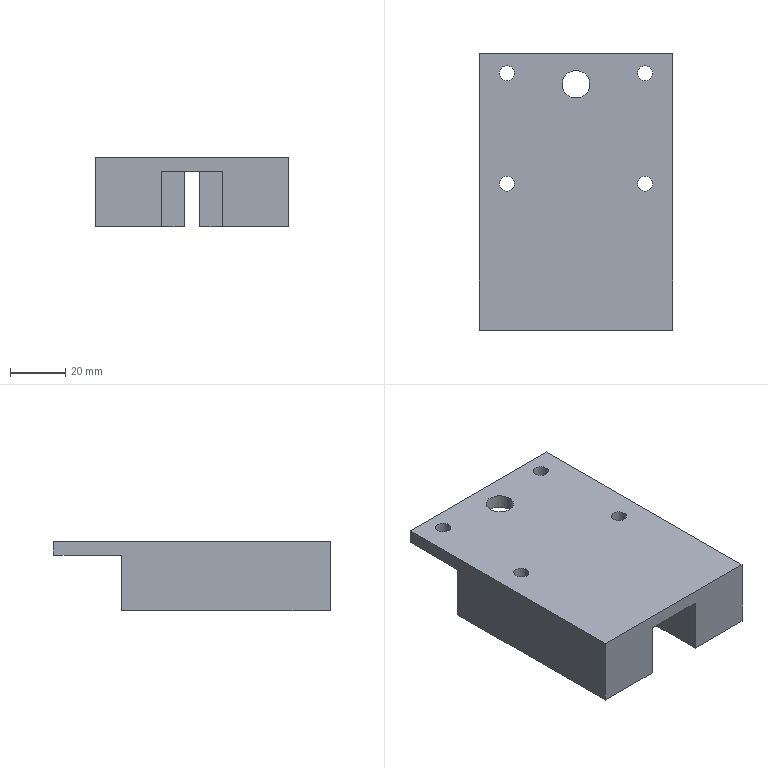Part | SolidWorks | features BaseBody 1 | 1 solid | 52 faces | box 70 x 100 x 25 mm | volume 106773 mm3 | plane 28 | cylinder 24 | commonest cylinder face diameters 5.5 x11 4.3 x4 9.5 x4 6 x3 10 x2